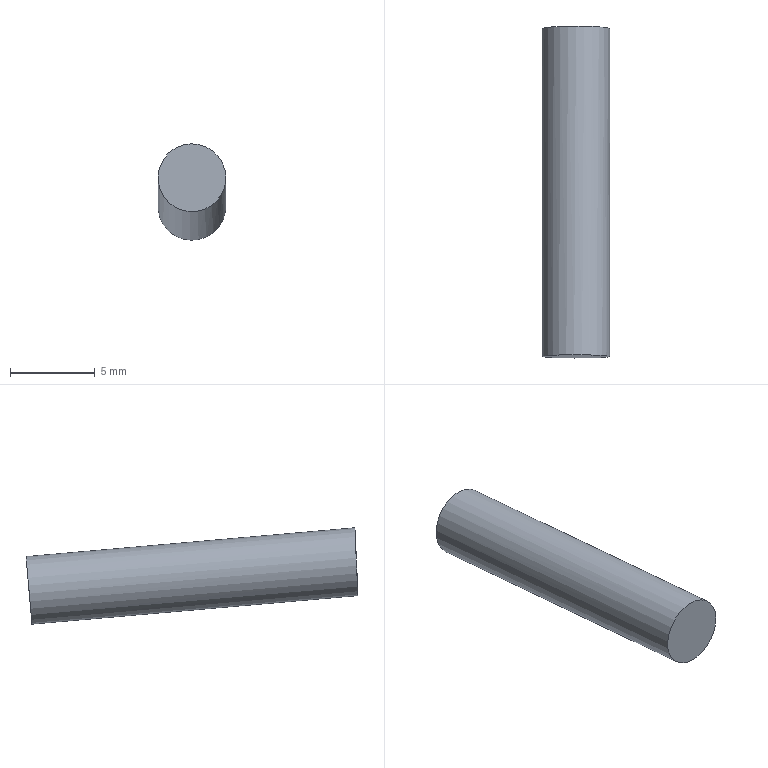Part | NX | features solid 2 | 1 solid | 3 faces | box 4 x 19.548 x 5.679 mm | volume 243.233 mm3 | plane 2 | cylinder 1 | commonest cylinder face diameters 4 x1
STEP:
#1=CARTESIAN_POINT('',(181.288,-26.618,-30.934));
#2=VERTEX_POINT('',#1);
#3=CARTESIAN_POINT('',(181.288,-26.792,-32.926));
#4=DIRECTION('',(0.,-0.9962,0.08716));
#5=DIRECTION('',(0.,0.08716,0.9962));
#6=AXIS2_PLACEMENT_3D('',#3,#4,#5);
#7=CIRCLE('',#6,2.);
#8=EDGE_CURVE('',#2,#2,#7,.T.);
#9=ORIENTED_EDGE('',*,*,#8,.F.);
#10=EDGE_LOOP('',(#9));
#11=FACE_BOUND('',#10,.T.);
#12=CARTESIAN_POINT('',(181.288,-26.792,-32.926));
#13=DIRECTION('',(0.,0.9962,-0.08716));
#14=DIRECTION('',(0.,-0.08716,-0.9962));
#15=AXIS2_PLACEMENT_3D('',#12,#13,#14);
#16=PLANE('',#15);
#17=ADVANCED_FACE('',(#11),#16,.T.);
#18=CARTESIAN_POINT('',(181.194,-46.165,-33.237));
#19=VERTEX_POINT('',#18);
#20=CARTESIAN_POINT('',(181.288,-46.074,-31.239));
#21=DIRECTION('',(0.001957,0.999,-0.04546));
#22=DIRECTION('',(-0.04675,-0.04532,-0.9979));
#23=AXIS2_PLACEMENT_3D('',#20,#21,#22);
#24=ELLIPSE('',#23,2.002,2.);
#25=EDGE_CURVE('',#19,#19,#24,.T.);
#26=ORIENTED_EDGE('',*,*,#25,.F.);
#27=EDGE_LOOP('',(#26));
#28=FACE_BOUND('',#27,.T.);
#29=CARTESIAN_POINT('',(128.811,-48.589,-88.763));
#30=DIRECTION('',(0.001957,0.999,-0.04546));
#31=DIRECTION('',(0.06617,0.04523,0.9968));
#32=AXIS2_PLACEMENT_3D('',#29,#30,#31);
#33=PLANE('',#32);
#34=ADVANCED_FACE('',(#28),#33,.F.);
#35=ORIENTED_EDGE('',*,*,#8,.T.);
#36=EDGE_LOOP('',(#35));
#37=FACE_BOUND('',#36,.T.);
#38=ORIENTED_EDGE('',*,*,#25,.T.);
#39=EDGE_LOOP('',(#38));
#40=FACE_BOUND('',#39,.T.);
#41=CARTESIAN_POINT('',(181.288,-46.716,-31.183));
#42=DIRECTION('',(0.,0.9962,-0.08716));
#43=DIRECTION('',(0.,-0.08716,-0.9962));
#44=AXIS2_PLACEMENT_3D('',#41,#42,#43);
#45=CYLINDRICAL_SURFACE('',#44,2.);
#46=ADVANCED_FACE('',(#37,#40),#45,.T.);
#47=CLOSED_SHELL('',(#17,#34,#46));
#48=MANIFOLD_SOLID_BREP('',#47);
#49=(LENGTH_UNIT()NAMED_UNIT(*)SI_UNIT(.MILLI.,.METRE.));
#50=UNCERTAINTY_MEASURE_WITH_UNIT(LENGTH_MEASURE(0.00001),#49,'','');
#51=(NAMED_UNIT(*)PLANE_ANGLE_UNIT()SI_UNIT($,.RADIAN.));
#52=(NAMED_UNIT(*)SI_UNIT($,.STERADIAN.)SOLID_ANGLE_UNIT());
#53=(GEOMETRIC_REPRESENTATION_CONTEXT(3)GLOBAL_UNCERTAINTY_ASSIGNED_CONTEXT((#50))GLOBAL_UNIT_ASSIGNED_CONTEXT((#49,#51,#52))REPRESENTATION_CONTEXT('',''));
#54=ADVANCED_BREP_SHAPE_REPRESENTATION('',(#48),#53);